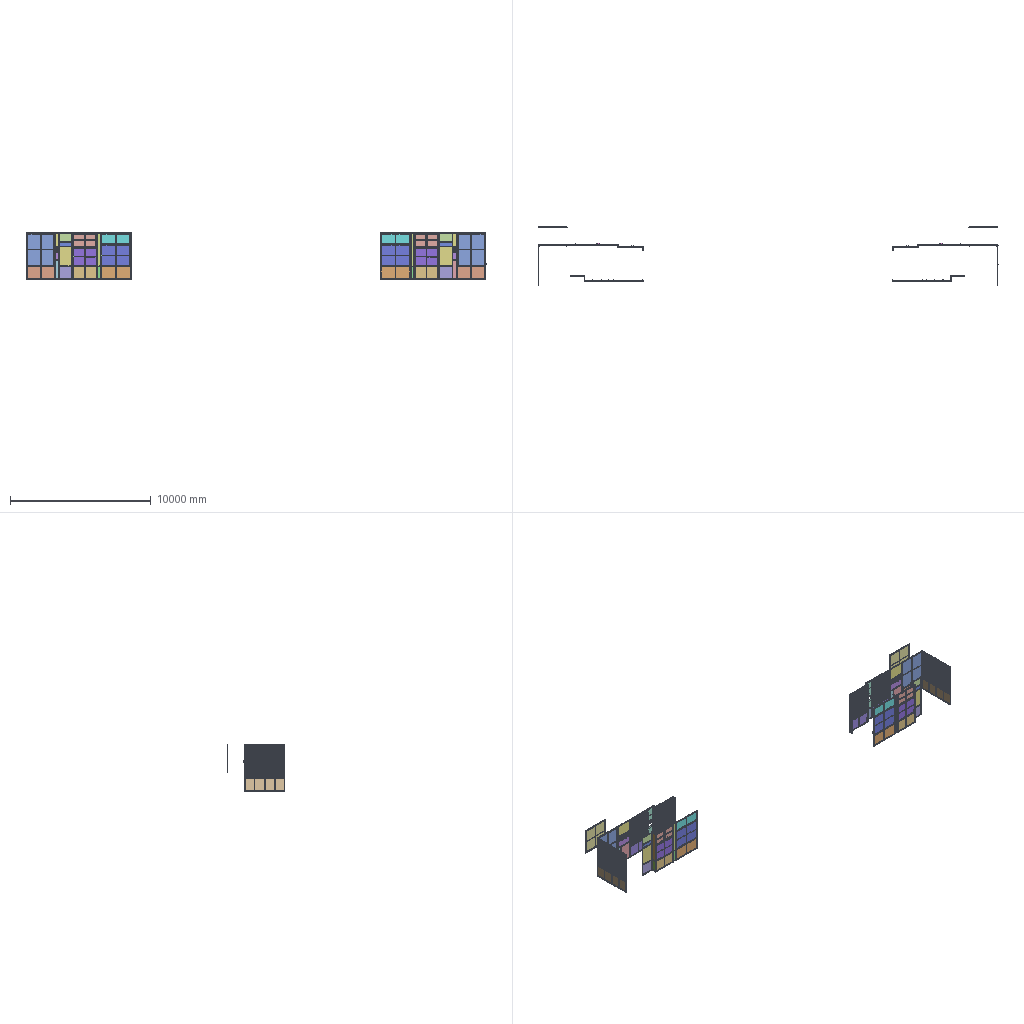Assembly | SolidWorks | 265 different items | 5997 placed | box 32704 x 4120 x 3280 mm
Parts list (item | name | quantity | parent item | size | volume | features):
1 | (subassembly) | x2 | in 40 | 1516 x 97 x 1065 mm | 8783731 mm3 | features ReferencePattern 4, CompositeCurve 1, DerivedHolePattern 1, LocalLPattern 1
2 | (subassembly) | x2 | in 40 | 722 x 54 x 1043 mm | 4219940 mm3 | features ReferencePattern 5, LocalLPattern 1
3 | (subassembly) | x2 | in 40 | 722 x 38 x 1043 mm | 4217360 mm3 | features ReferencePattern 5, LocalLPattern 1
4 | (subassembly) | x2 | - | - | - | -
5 | (subassembly) | x4 | in 4, 24 | - | 15054110 mm3 | features ReferencePattern 36, LocalLPattern 5, MirrorCompFeat 1
6 | (subassembly) | x4 | in 4, 24 | - | - | features ReferencePattern 178, LocalLPattern 10, MirrorCompFeat 4, CompositeCurve 1
7 | (subassembly) | x2 | - | - | 10335733 mm3 | features ReferencePattern 12, LocalLPattern 4
8 | (subassembly) | x2 | - | - | 7266370 mm3 | features ReferencePattern 12, LocalLPattern 4
9 | (subassembly) | x2 | - | - | 21498613 mm3 | -
10 | (subassembly) | x2 | in 9 | - | 21498613 mm3 | features ReferencePattern 30, LocalLPattern 10, MirrorCompFeat 1
11 | (subassembly) | x2 | - | - | 41950678 mm3 | -
12 | (subassembly) | x2 | in 11 | - | 17564416 mm3 | features ReferencePattern 19, LocalLPattern 3, DerivedHolePattern 2
13 | (subassembly) | x2 | in 11 | 2296 x 114.543 x 991.55 mm | 12200814 mm3 | features LocalLPattern 3, ReferencePattern 2, CompositeCurve 1
14 | (subassembly) | x2 | in 11 | 2296 x 97 x 991.55 mm | 12185495 mm3 | features LocalLPattern 2, ReferencePattern 1
15 | (subassembly) | x2 | - | - | 24877160 mm3 | -
16 | (subassembly) | x2 | in 15 | - | 5346170 mm3 | features ReferencePattern 13, DerivedHolePattern 3, LocalLPattern 2
17 | (subassembly) | x2 | in 15 | 1832 x 15 x 970 mm | 9765548 mm3 | features ReferencePattern 2, LocalLPattern 1
18 | (subassembly) | x2 | in 15 | 1832 x 15 x 970 mm | 9765539 mm3 | features ReferencePattern 2, LocalLPattern 1
19 | (subassembly) | x2 | - | - | 9752547 mm3 | -
20 | (subassembly) | x4 | - | - | 36484784 mm3 | -
21 | (subassembly) | x4 | in 20 | - | 13059635 mm3 | features ReferencePattern 57, LocalLPattern 5
22 | (subassembly) | x4 | in 20 | - | 23425150 mm3 | features ReferencePattern 138, LocalLPattern 9, MirrorCompFeat 4
23 | (subassembly) | x2 | - | - | 6905268 mm3 | features ReferencePattern 12, LocalLPattern 4
24 | (subassembly) | x2 | - | - | - | -
25 | (subassembly) | x2 | - | - | 7789967 mm3 | features ReferencePattern 12, LocalLPattern 4
26 | (subassembly) | x2 | - | - | 39443592 mm3 | -
27 | (subassembly) | x2 | in 26 | - | 16846770 mm3 | features ReferencePattern 45, LocalLPattern 6, MirrorCompFeat 5, CompositeCurve 3
28 | (subassembly) | x2 | in 19 | - | 7457075 mm3 | features ReferencePattern 8, LocalLPattern 2
29 | (subassembly) | x2 | in 26 | 1296 x 114.543 x 856.55 mm | 6140748 mm3 | features LocalLPattern 3, ReferencePattern 3, CompositeCurve 2
30 | (subassembly) | x2 | in 26 | 1296 x 97 x 857.775 mm | 6137895 mm3 | features LocalLPattern 2, ReferencePattern 2
31 | (subassembly) | x4 | in 26 | 852 x 78 x 956 mm | 5159135 mm3 | features ReferencePattern 28, LocalLPattern 5, MirrorCompFeat 2
32 | (subassembly) | x458 | in 5, 7, 8, 10, 12, 16, 21, 23, 25, 27, 28, 31, 39, 41 | 45.75 x 28.75 x 16 mm | 4951 mm3 | -
33 | (subassembly) | x1 | - | 46.643 x 46.639 x 38 mm | 6782 mm3 | -
34 | (subassembly) | x16 | in 31, 39 | 62 x 12.05 x 82 mm | 23876 mm3 | -
35 | (subassembly) | x16 | in 6 | 11 x 45 x 115 mm | 44302 mm3 | -
36 | (subassembly) | x1 | - | 69.2 x 20.1 x 100 mm | 14261 mm3 | -
37 | (subassembly) | x16 | in 16, 21, 41 | - | - | -
38 | (subassembly) | x2 | in 19 | 560.594 x 2339 x 38 mm | 2295468 mm3 | features ReferencePattern 12, LocalLPattern 3
39 | (subassembly) | x2 | - | - | 27416958 mm3 | features ReferencePattern 79, LocalLPattern 15, MirrorCompFeat 6, CompositeCurve 2
40 | (subassembly) | x2 | - | - | 46606535 mm3 | -
41 | (subassembly) | x2 | in 40 | - | 20597906 mm3 | features ReferencePattern 98, LocalLPattern 9
42 | (subassembly) | x2 | in 40 | 1516 x 114.543 x 1065 mm | 8787872 mm3 | features ReferencePattern 5, LocalLPattern 3, CompositeCurve 1
43 | - | x4 | in 6 | 160 x 64 x 4 mm | 39767 mm3 | features HoleWzd 2, Extrusion 1, Fillet 1
44 | - | x8 | in 12 | 14 x 20.3 x 907 mm | 46181 mm3 | features BaseBody 1, ICE 1, MoveFace 1
45 | - | x8 | in 8 | 14 x 20.3 x 95 mm | 4837 mm3 | features BaseBody 1, ICE 1, MoveFace 1
46 | - | x8 | in 41 | 14 x 20.3 x 980 mm | 49897 mm3 | features BaseBody 1, ICE 1, MoveFace 1
47 | - | x2 | in 29 | 30 x 15 x 1236 mm | 297813 mm3 | features HoleWzd 3, BaseBody 1, MoveFace 1
48 | - | x4 | in 29, 30 | 30 x 15 x 1236 mm | 297203 mm3 | features HoleWzd 3, BaseBody 1, MoveFace 1
49 | - | x2 | in 30 | 30 x 15 x 1236 mm | 297813 mm3 | features BaseBody 1, HoleWzd 1, MoveFace 1
50 | - | x4 | in 1, 42 | 30 x 15 x 1456 mm | 350164 mm3 | features HoleWzd 3, BaseBody 1, MoveFace 1
51 | - | x4 | in 1, 42 | 30 x 15 x 1456 mm | 351142 mm3 | features BaseBody 1, HoleWzd 1, MoveFace 1
52 | - | x4 | in 17, 18 | 30 x 15 x 1772 mm | 426374 mm3 | features HoleWzd 3, BaseBody 1, MoveFace 1
53 | - | x4 | in 17, 18 | 30 x 15 x 1772 mm | 427079 mm3 | features BaseBody 1, HoleWzd 1, MoveFace 1
54 | - | x8 | in 6 | 40 x 40 x 4 mm | 5920 mm3 | features HoleWzd 3, Extrusion 1, Fillet 1
55 | - | x4 | in 13, 14 | 30 x 15 x 2236 mm | 538276 mm3 | features HoleWzd 3, BaseBody 1, MoveFace 1
56 | - | x1 | - | 30 x 15 x 2236 mm | 538276 mm3 | features HoleWzd 3, BaseBody 1, MoveFace 1
57 | - | x1 | - | 30 x 15 x 2236 mm | 538276 mm3 | features HoleWzd 3, BaseBody 1, MoveFace 1
58 | - | x1 | - | 30 x 15 x 2236 mm | 538710 mm3 | features BaseBody 1, HoleWzd 1, MoveFace 1
59 | - | x4 | in 13, 14 | 30 x 15 x 2236 mm | 538982 mm3 | features BaseBody 1, HoleWzd 1, MoveFace 1
60 | - | x1 | - | 30 x 15 x 630 mm | 151936 mm3 | features BaseBody 1, MoveFace 1
61 | - | x4 | in 2, 3 | 30 x 15 x 662 mm | 159462 mm3 | features BaseBody 1, HoleWzd 1, MoveFace 1
62 | - | x4 | in 2, 3 | 30 x 15 x 662 mm | 159654 mm3 | features BaseBody 1, MoveFace 1
63 | - | x12 | in 29, 30 | 30 x 15 x 775 mm | 186906 mm3 | features BaseBody 1, MoveFace 1
64 | - | x1 | - | 30 x 15 x 791 mm | 190764 mm3 | features BaseBody 1, MoveFace 1
65 | - | x12 | in 12, 27, 41 | 45 x 26 x 108 mm | 14308 mm3 | features HoleWzd 2, Fillet 1, FlatPattern 1, SMBaseFlange 1, SheetMetal 1
66 | - | x4 | in 13, 14 | 30 x 15 x 910 mm | 219062 mm3 | features BaseBody 1, HoleWzd 1, MoveFace 1
67 | - | x20 | in 13, 14, 17, 18 | 30 x 15 x 910 mm | 219464 mm3 | features BaseBody 1, MoveFace 1
68 | - | x20 | in 1, 2, 3, 42 | 30 x 15 x 983 mm | 237069 mm3 | features BaseBody 1, MoveFace 1
69 | - | x4 | in 39 | 40 x 40 x 1350 mm | 790915 mm3 | features BaseBody 1, HoleWzd 1, MoveFace 1
70 | - | x20 | in 5, 21, 24 | 40 x 40 x 3280 mm | 1969669 mm3 | features HoleWzd 2, Extrusion 1
71 | - | x8 | in 39 | 40 x 40 x 1146 mm | 670131 mm3 | features BaseBody 1, HoleWzd 1, MoveFace 1
72 | - | x6 | in 23 | 40 x 40 x 135 mm | 71545 mm3 | features BaseBody 1, HoleWzd 1, MoveFace 1
73 | - | x4 | in 21 | 40 x 40 x 1360 mm | 796835 mm3 | features BaseBody 1, HoleWzd 1, MoveFace 1
74 | - | x6 | in 8 | 40 x 40 x 155 mm | 83386 mm3 | features BaseBody 1, HoleWzd 1, MoveFace 1
75 | - | x8 | in 27 | 40 x 40 x 1650 mm | 968537 mm3 | features BaseBody 1, HoleWzd 1, MoveFace 1
76 | - | x6 | in 1, 14, 30 | 52 x 17 x 50 mm | 6238 mm3 | features HoleWzd 2, Fillet 1, FlatPattern 1, SMBaseFlange 1, SheetMetal 1
77 | - | x4 | in 5 | 40 x 40 x 1682 mm | 987483 mm3 | features BaseBody 1, HoleWzd 1, MoveFace 1
78 | - | x6 | in 25 | 40 x 40 x 184 mm | 100557 mm3 | features BaseBody 1, HoleWzd 1, MoveFace 1
79 | - | x10 | in 12, 16 | 40 x 40 x 1920 mm | 1128397 mm3 | features BaseBody 1, HoleWzd 1, MoveFace 1
80 | - | x2 | in 39 | 40 x 40 x 1930 mm | 1139883 mm3 | features HoleWzd 4, MoveFace 2, BaseBody 1
81 | - | x4 | in 16 | 40 x 40 x 1930 mm | 1140355 mm3 | features HoleWzd 3, BaseBody 1, MoveFace 1
82 | - | x8 | in 41 | 40 x 40 x 2066 mm | 1214839 mm3 | features BaseBody 1, HoleWzd 1, MoveFace 1
83 | - | x2 | in 39 | 40 x 40 x 308 mm | 173974 mm3 | features BaseBody 1, HoleWzd 1, MoveFace 1
84 | - | x6 | in 7 | 40 x 40 x 325 mm | 184039 mm3 | features BaseBody 1, HoleWzd 1, MoveFace 1
85 | - | x24 | in 7, 8, 23, 25, 28, 41 | 40 x 40 x 3280 mm | 1939169 mm3 | features HoleWzd 4, 3DProfileFeature 1, BaseBody 1, MoveFace 1
86 | - | x2 | in 39 | 40 x 40 x 3280 mm | 1938394 mm3 | features HoleWzd 4, BaseBody 1, MoveFace 1
87 | - | x6 | in 13, 29, 42 | 68 x 17 x 50 mm | 7802 mm3 | features HoleWzd 2, Fillet 1, FlatPattern 1, SMBaseFlange 1, SheetMetal 1
88 | - | x2 | in 27 | 40 x 40 x 3280 mm | 1938394 mm3 | features HoleWzd 6, BaseBody 1, MoveFace 1
89 | - | x2 | in 27 | 40 x 40 x 3280 mm | 1938394 mm3 | features HoleWzd 6, BaseBody 1, MoveFace 1
90 | - | x4 | in 12 | 40 x 40 x 3280 mm | 1940425 mm3 | features HoleWzd 2, BaseBody 1, MoveFace 1
91 | - | x6 | in 28 | 40 x 40 x 536 mm | 308966 mm3 | features BaseBody 1, HoleWzd 1, MoveFace 1
92 | - | x2 | in 39 | 40 x 40 x 798 mm | 464090 mm3 | features BaseBody 1, HoleWzd 1, MoveFace 1
93 | - | x14 | in 5, 12, 21, 27, 41 | 40 x 40 x 846 mm | 492509 mm3 | features BaseBody 1, HoleWzd 1, MoveFace 1
94 | - | x10 | in 10 | 40 x 40 x 880 mm | 512640 mm3 | features BaseBody 1, HoleWzd 1, MoveFace 1
95 | - | x8 | in 39 | 40 x 40 x 339 mm | 146697 mm3 | features BaseBody 1, MoveFace 1
96 | - | x12 | in 39 | 40 x 40 x 488 mm | 205502 mm3 | features BaseBody 1, HoleWzd 1, MoveFace 1
97 | - | x12 | in 31 | 40 x 40 x 740 mm | 314551 mm3 | features BaseBody 1, HoleWzd 1, MoveFace 1
98 | - | x8 | in 27, 39 | 70 x 54 x 82 mm | 19533 mm3 | features HoleWzd 3, EdgeFlange 2, Chamfer 1, Fillet 1, FlatPattern 1, MirrorPattern 1, SMBaseFlange 1, SheetMetal 1
99 | - | x8 | in 31 | 40 x 40 x 956 mm | 413693 mm3 | features BaseBody 1, MoveFace 1
100 | - | x8 | in 21 | 40 x 40 x 1360 mm | 721762 mm3 | features BaseBody 1, HoleWzd 1, MoveFace 1
101 | - | x1 | - | 40 x 40 x 155 mm | 83065 mm3 | features BaseBody 1, HoleWzd 1, MoveFace 1
102 | - | x8 | in 5 | 40 x 40 x 1682 mm | 894323 mm3 | features BaseBody 1, HoleWzd 1, MoveFace 1
103 | - | x1 | - | 40 x 40 x 1762 mm | 942816 mm3 | features BaseBody 1, HoleWzd 1, MoveFace 1
104 | - | x1 | - | 40 x 40 x 2150 mm | 1150023 mm3 | features BaseBody 1, HoleWzd 1, MoveFace 1
105 | - | x1 | - | 40 x 40 x 2154 mm | 1154336 mm3 | features BaseBody 1, HoleWzd 1, MoveFace 1
106 | - | x32 | in 6, 22 | 40 x 40 x 2310 mm | 1236491 mm3 | features BaseBody 1
107 | - | x1 | - | 40 x 40 x 255 mm | 136655 mm3 | features BaseBody 1, HoleWzd 1, MoveFace 1
108 | - | x4 | in 10 | 40 x 40 x 3280 mm | 1939269 mm3 | features HoleWzd 3, BaseBody 1, MoveFace 1
109 | - | x8 | in 27, 39 | 42 x 25 x 50 mm | 6162 mm3 | features HoleWzd 3, EdgeFlange 2, Chamfer 1, Fillet 1, FlatPattern 1, MirrorPattern 1, SMBaseFlange 1, SheetMetal 1
110 | - | x8 | in 22 | 40 x 40 x 588 mm | 315111 mm3 | features BaseBody 1, MoveFace 1
111 | - | x20 | in 22 | 40 x 40 x 588 mm | 315111 mm3 | features BaseBody 1, MoveFace 1
112 | - | x28 | in 6 | 40 x 40 x 749 mm | 401392 mm3 | features BaseBody 1, MoveFace 1
113 | - | x1 | - | 40 x 40 x 757 mm | 405679 mm3 | features BaseBody 1, MoveFace 1
114 | - | x16 | in 22 | 60 x 38 x 3 mm | 6476 mm3 | features BaseBody 1
115 | - | x32 | in 35 | 45 x 11 x 113 mm | 18493 mm3 | features BaseBody 1
116 | - | x16 | in 35 | 9 x 9 x 115 mm | 7316 mm3 | features BaseBody 1
117 | - | x160 | in 1, 2, 3, 13, 14, 17, 18, 29, 30, 42 | 10.5 x 10.5 x 19.3 mm | 617.652 mm3 | features BaseBody 1
118 | - | x4 | in 27 | 11.6 x 1.2 x 11.6 mm | 88.216 mm3 | features Extrusion 1
119 | - | x8 | in 41 | 17.5 x 34 x 40 mm | 3554 mm3 | features HoleWzd 2, Fillet 1, FlatPattern 1, SMBaseFlange 1, SheetMetal 1
120 | - | x40 | in 12, 16, 27, 41 | 7 x 7 x 0.5 mm | 15.221 mm3 | features Revolution 1
121 | - | x16 | in 2, 3 | 9 x 9 x 0.8 mm | 39.276 mm3 | features Revolution 1
122 | - | x124 | in 5, 12, 16, 21, 27, 41 | 10 x 10 x 1 mm | 56.478 mm3 | features Revolution 1
123 | - | x32 | in 22 | 12.5 x 12.5 x 1.6 mm | 144.878 mm3 | features Revolution 1
124 | - | x96 | in 6 | 15 x 8.5 x 20 mm | 1520 mm3 | features BaseBody 1
125 | - | x32 | in 22 | 12.197 x 12.2 x 1.5 mm | 128.674 mm3 | features ICE 1, Revolution 1
126 | - | x8 | in 31, 39 | 107 x 38 x 20.5 mm | 23344 mm3 | features BaseBody 1
127 | - | x12 | in 12, 27, 41 | - | - | features BaseBody 30, RefSurface 1
128 | - | x12 | in 1, 13, 14, 29, 30, 42 | 35.586 x 51.386 x 50.3 mm | 17360 mm3 | features BaseBody 15
129 | - | x4 | in 41 | 1009 x 842 x 5 mm | 4247890 mm3 | features Extrusion 1, HoleWzd 1
130 | - | x2 | in 38 | 533 x 2311 x 38 mm | 2271037 mm3 | features SMWeldBead 4, EdgeFlange 2, HoleWzd 2, BossThin 1, FlatPattern 1, ICE 1, SMBaseFlange 1, SheetMetal 1
131 | - | x16 | in 22 | 584 x 1091 x 5 mm | 3185720 mm3 | features Extrusion 1, HoleWzd 1
132 | - | x16 | in 6 | 745 x 1091 x 5 mm | 4063975 mm3 | features Extrusion 1, HoleWzd 1
133 | - | x1 | - | 646 x 1119 x 5 mm | 3614370 mm3 | features Extrusion 1
134 | - | x1 | - | 807 x 1119 x 5 mm | 4515165 mm3 | features Extrusion 1
135 | - | x8 | in 13, 14 | 926 x 1119 x 5 mm | 5180970 mm3 | features Extrusion 1
136 | - | x2 | in 39 | 1142 x 513 x 5 mm | 2929230 mm3 | features Extrusion 1, HoleWzd 1
137 | - | x2 | in 39 | 1142 x 906 x 5 mm | 5173260 mm3 | features Extrusion 1, HoleWzd 1
138 | - | x2 | in 23 | 131 x 2310 x 5 mm | 1513050 mm3 | features Extrusion 1, HoleWzd 1
139 | - | x2 | in 23 | 131 x 842 x 5 mm | 551510 mm3 | features Extrusion 1, HoleWzd 1
140 | - | x2 | in 8 | 151 x 2310 x 5 mm | 1744050 mm3 | features Extrusion 1, HoleWzd 1
141 | - | x16 | in 6 | 1144 x 813 x 7 mm | 815811 mm3 | features ICE 5, Extrusion 1, HoleWzd 1, WeldmentFeature 1
142 | - | x2 | in 8 | 151 x 842 x 5 mm | 635710 mm3 | features Extrusion 1, HoleWzd 1
143 | - | x2 | in 25 | 180 x 2310 x 5 mm | 2079000 mm3 | features Extrusion 1, HoleWzd 1
144 | - | x2 | in 25 | 180 x 842 x 5 mm | 757800 mm3 | features Extrusion 1, HoleWzd 1
145 | - | x2 | in 39 | 304 x 1306 x 5 mm | 1985120 mm3 | features Extrusion 1, HoleWzd 1
146 | - | x2 | in 7 | 321 x 2310 x 5 mm | 3707550 mm3 | features Extrusion 1, HoleWzd 1
147 | - | x2 | in 7 | 321 x 842 x 5 mm | 1351410 mm3 | features Extrusion 1, HoleWzd 1
148 | - | x8 | in 39 | 484 x 105 x 5 mm | 254100 mm3 | features Extrusion 1, HoleWzd 1
149 | - | x2 | in 28 | 532 x 842 x 5 mm | 2239720 mm3 | features Extrusion 1, HoleWzd 1
150 | - | x8 | in 29, 30 | 619 x 791 x 5 mm | 2448145 mm3 | features Extrusion 1
151 | - | x8 | in 21 | 656 x 842 x 5 mm | 2761760 mm3 | features Extrusion 1, HoleWzd 1
152 | - | x16 | in 22 | 1143 x 652 x 7 mm | 701424 mm3 | features ICE 5, Extrusion 1, HoleWzd 1, WeldmentFeature 1
153 | - | x4 | in 2, 3 | 997 x 678 x 5 mm | 3379830 mm3 | features Extrusion 1
154 | - | x8 | in 31 | 414 x 736 x 5 mm | 1523520 mm3 | features Extrusion 1, HoleWzd 1
155 | - | x2 | in 39 | 794 x 1306 x 5 mm | 5184820 mm3 | features Extrusion 1, HoleWzd 1
156 | - | x4 | in 27 | 801 x 842 x 5 mm | 3372210 mm3 | features Extrusion 1, HoleWzd 1
157 | - | x8 | in 5 | 817 x 842 x 5 mm | 3439570 mm3 | features Extrusion 1, HoleWzd 1
158 | - | x2 | in 10 | 876 x 1360 x 5 mm | 5956800 mm3 | features Extrusion 1, HoleWzd 1
159 | - | x2 | in 10 | 876 x 291 x 5 mm | 1274580 mm3 | features Extrusion 1, HoleWzd 1
160 | - | x2 | in 10 | 876 x 571 x 5 mm | 2500980 mm3 | features Extrusion 1, HoleWzd 1
161 | - | x2 | in 10 | 876 x 842 x 5 mm | 3687960 mm3 | features Extrusion 1, HoleWzd 1
162 | - | x8 | in 17, 18 | 926 x 887 x 5 mm | 4106810 mm3 | features Extrusion 1
163 | - | x8 | in 27, 39 | 16.002 x 50.042 x 18.313 mm | 6537 mm3 | features BaseBody 8
164 | - | x4 | in 12 | 936 x 842 x 5 mm | 3940560 mm3 | features Extrusion 1, HoleWzd 1
165 | - | x8 | in 1, 42 | 999 x 729 x 5 mm | 3641355 mm3 | features Extrusion 1
166 | - | x4 | in 27 | 10 x 4.5 x 6 mm | 142.178 mm3 | features ICE 2, Extrusion 1, Fillet 1, RevCut 1
167 | - | x4 | in 27 | 19 x 7.5 x 7.999 mm | 677.198 mm3 | features ICE 2, Extrusion 1, RevCut 1
168 | - | x12 | in 1, 13, 14, 29, 30, 42 | 18 x 135 x 30 mm | 20354 mm3 | features BaseBody 1
169 | - | x12 | in 14, 29, 30 | 8 x 8 x 20 mm | 286.49 mm3 | features BaseBody 1
170 | - | x40 | in 1, 2, 3, 13, 14, 17, 18, 29, 30, 42 | 32 x 32 x 15 mm | 8367 mm3 | features BaseBody 1
171 | - | x26 | in 6, 27, 39 | 55 x 14.5 x 18 mm | 8175 mm3 | features BaseBody 1
172 | - | x20 | in 12, 16, 27, 41 | 17 x 15 x 50 mm | 8082 mm3 | features BaseBody 1
173 | - | x4 | in 6 | 16.3 x 18.3 x 16.3 mm | 1833 mm3 | features BaseBody 1
174 | - | x8 | in 27, 39 | 16.008 x 126.481 x 28.318 mm | 9351 mm3 | features BaseBody 7
175 | - | x1 | - | 8 x 1328 x 777 mm | 322628 mm3 | features BaseBody 1, ICE 1, MirrorPattern 1
176 | - | x1 | - | 8 x 742 x 777 mm | 178056 mm3 | features BaseBody 1, ICE 1, MirrorPattern 1
177 | - | x4 | in 27 | 33.5 x 13.5 x 1650 mm | 308881 mm3 | features BaseBody 1, HoleWzd 1, ICE 1, MoveFace 1
178 | - | x4 | in 12 | 33.5 x 13.5 x 1920 mm | 359220 mm3 | features ICE 2, BaseBody 1, HoleWzd 1, MoveFace 1
179 | - | x4 | in 16 | 33.5 x 13.5 x 1920 mm | 359220 mm3 | features ICE 2, BaseBody 1, HoleWzd 1, MoveFace 1
180 | - | x4 | in 6 | - | 237710 mm3 | features BaseBody 17, ICE 1
181 | - | x8 | in 41 | 33.5 x 13.5 x 2066 mm | 386658 mm3 | features ICE 2, BaseBody 1, HoleWzd 1, MoveFace 1
182 | - | x40 | in 1, 2, 3, 13, 14, 17, 18, 29, 30, 42 | 32 x 32 x 15 mm | 8036 mm3 | features BaseBody 1
183 | - | x4 | in 6 | - | 135185 mm3 | features BaseBody 17
184 | - | x8 | in 10 | 13.8 x 7.5 x 8 mm | 622.996 mm3 | features BaseBody 1
185 | - | x260 | in 5, 6, 12, 21, 22, 27, 39, 41 | 19.5 x 6 x 8 mm | 667.11 mm3 | features BaseBody 1
186 | - | x550 | in 5, 12, 21, 31, 32, 39, 41 | 19.5 x 6 x 8 mm | 631.457 mm3 | features BaseBody 1
187 | - | x174 | in 5, 7, 8, 10, 12, 16, 21, 23, 25, 28, 31, 38, 39, 41 | 13.001 x 8.797 x 21 mm | 1304 mm3 | features BaseBody 1
188 | - | x1 | - | - | - | features RefSurface 120
189 | - | x1 | - | 41 x 41 x 38 mm | 6489 mm3 | features BaseBody 1
190 | - | x16 | in 34 | 36.75 x 12.05 x 79 mm | 10360 mm3 | features BaseBody 1
191 | - | x16 | in 34 | 7 x 7 x 82 mm | 3156 mm3 | features BaseBody 1
192 | - | x16 | in 34 | 36.75 x 12.05 x 79 mm | 10360 mm3 | features BaseBody 1
193 | - | x1 | - | 69.2 x 20 x 100 mm | 10290 mm3 | features BaseBody 1
194 | - | x1 | - | 69.2 x 7 x 25.2 mm | 3971 mm3 | features BaseBody 1
195 | - | x2 | in 39 | 9.5 x 13.5 x 140 mm | 13278 mm3 | features BaseBody 1
196 | - | x120 | in 5, 12, 16, 21, 27, 41 | 5.5 x 6.351 x 2.4 mm | 50.752 mm3 | features BaseBody 1
197 | - | x56 | in 12, 16, 27, 41 | 7 x 8.083 x 3.2 mm | 107.56 mm3 | features BaseBody 1
198 | - | x2 | in 27 | 8 x 9.238 x 4 mm | 165.049 mm3 | features BaseBody 1
199 | - | x1 | - | 39 x 25 x 60 mm | 7010 mm3 | features HoleWzd 2, Chamfer 1, FlatPattern 1, SMBaseFlange 1, SheetMetal 1
200 | - | x40 | in 12, 16, 27, 41 | 5.5 x 5.5 x 11 mm | 117.558 mm3 | features ICE 2, Chamfer 1, RevCut 1, Revolution 1
201 | - | x16 | in 41 | 7 x 7 x 16 mm | 285.079 mm3 | features ICE 2, Chamfer 1, RevCut 1, Revolution 1
202 | - | x80 | in 1, 2, 3, 13, 14, 29, 30, 42 | 7 x 7 x 12 mm | 234.462 mm3 | features ICE 3, Chamfer 1, RevCut 1, Revolution 1
203 | - | x292 | in 5, 6, 12, 16, 21, 27, 39, 41 | 17 x 8.5 x 8.5 mm | 477.486 mm3 | features ICE 1, RevCut 1, Revolution 1
204 | - | x24 | in 38 | 18 x 10 x 10 mm | 732.461 mm3 | features ICE 1, RevCut 1, Revolution 1
205 | - | x32 | in 22 | 22 x 10 x 10 mm | 845.558 mm3 | features ICE 1, RevCut 1, Revolution 1
206 | - | x16 | in 31, 39 | 10 x 10 x 24 mm | 898.677 mm3 | features Chamfer 2, ICE 2, RevCut 1, Revolution 1
207 | - | x16 | in 13, 14, 17, 18 | 10 x 10 x 36 mm | 1238 mm3 | features Chamfer 2, ICE 2, RevCut 1, Revolution 1
208 | - | x124 | in 5, 7, 8, 10, 12, 16, 21, 23, 25, 28, 39, 41 | 10 x 10 x 46 mm | 1521 mm3 | features Chamfer 2, ICE 2, RevCut 1, Revolution 1
209 | - | x72 | in 6, 22 | 13 x 13 x 48 mm | 2916 mm3 | features Chamfer 2, ICE 2, RevCut 1, Revolution 1
210 | - | x1 | - | 23 x 25 x 60 mm | 5085 mm3 | features HoleWzd 2, Chamfer 1, FlatPattern 1, SMBaseFlange 1, SheetMetal 1
211 | - | x40 | in 12, 16, 27, 41 | 8 x 8 x 10 mm | 162.002 mm3 | features BaseBody 1
212 | - | x1 | - | 10 x 10 x 12 mm | 304.022 mm3 | features BaseBody 1
213 | - | x48 | in 31, 39 | 12 x 12 x 15 mm | 531.654 mm3 | features BaseBody 1
214 | - | x48 | in 31, 39 | 12 x 12 x 25 mm | 814.397 mm3 | features BaseBody 1
215 | - | x212 | in 5, 6, 12, 16, 21, 22, 27, 41 | 12 x 12 x 12 mm | 460.573 mm3 | features Chamfer 1, ICE 1, Revolution 1
216 | - | x8 | in 27 | 17 x 8.5 x 8.5 mm | 492.043 mm3 | features ICE 1, Revolution 1
217 | - | x458 | in 32 | 10 x 10 x 31 mm | 1100 mm3 | features BaseBody 1
218 | - | x1 | - | 38 x 31 x 14.5 mm | 4841 mm3 | features BaseBody 1
219 | - | x8 | in 25 | 10.8 x 17.5 x 124 mm | 9771 mm3 | features MoveFace 2, BaseBody 1
220 | - | x4 | in 10 | 10.8 x 17.5 x 1358 mm | 107011 mm3 | features BaseBody 1, MoveFace 1
221 | - | x18 | in 2, 29, 42 | 39 x 17 x 40 mm | 4045 mm3 | features HoleWzd 2, FlatPattern 1, SMBaseFlange 1, SheetMetal 1
222 | - | x16 | in 7, 8, 23, 25 | 10.8 x 17.5 x 1171 mm | 92275 mm3 | features BaseBody 1, MoveFace 1
223 | - | x8 | in 7 | 10.8 x 17.5 x 265 mm | 20882 mm3 | features BaseBody 1, MoveFace 1
224 | - | x4 | in 28 | 10.8 x 17.5 x 476 mm | 37509 mm3 | features BaseBody 1, MoveFace 1
225 | - | x16 | in 21 | 10.8 x 17.5 x 627 mm | 49408 mm3 | features BaseBody 1, MoveFace 1
226 | - | x8 | in 23 | 10.8 x 17.5 x 75 mm | 5910 mm3 | features BaseBody 1, MoveFace 1
227 | - | x8 | in 27 | 10.8 x 17.5 x 774 mm | 60992 mm3 | features BaseBody 1, MoveFace 1
228 | - | x24 | in 5, 12, 21, 41 | 10.8 x 17.5 x 786 mm | 61937 mm3 | features BaseBody 1, MoveFace 1
229 | - | x24 | in 5, 27 | 10.8 x 17.5 x 788 mm | 62095 mm3 | features BaseBody 1, MoveFace 1
230 | - | x16 | in 10 | 10.8 x 17.5 x 820 mm | 64616 mm3 | features BaseBody 1, MoveFace 1
231 | - | x48 | in 5, 7, 8, 10, 12, 21, 23, 25, 28, 41 | 10.8 x 17.5 x 840 mm | 66192 mm3 | features BaseBody 1, MoveFace 1
232 | - | x20 | in 12, 16, 27, 41 | 17.5 x 17 x 60 mm | 3562 mm3 | features HoleWzd 2, FlatPattern 1, SMBaseFlange 1, SheetMetal 1
233 | - | x8 | in 12 | 10.8 x 17.5 x 907 mm | 71472 mm3 | features BaseBody 1, MoveFace 1
234 | - | x8 | in 8 | 10.8 x 17.5 x 95 mm | 7486 mm3 | features MoveFace 2, BaseBody 1
235 | - | x8 | in 41 | 10.8 x 17.5 x 980 mm | 77225 mm3 | features BaseBody 1, MoveFace 1
236 | - | x8 | in 7 | 14 x 20.3 x 265 mm | 13493 mm3 | features MoveFace 2, BaseBody 1, ICE 1
237 | - | x8 | in 39 | 14 x 20.3 x 1088 mm | 55396 mm3 | features BaseBody 1, ICE 1, MoveFace 1
238 | - | x16 | in 39 | 14 x 20.3 x 108 mm | 5499 mm3 | features MoveFace 2, BaseBody 1, ICE 1
239 | - | x64 | in 6, 22 | 14 x 20.3 x 1090 mm | 55498 mm3 | features BaseBody 1, ICE 1, MoveFace 1
240 | - | x8 | in 25 | 14 x 20.3 x 124 mm | 6314 mm3 | features BaseBody 1, ICE 1, MoveFace 1
241 | - | x8 | in 39 | 14 x 20.3 x 1280 mm | 65172 mm3 | features BaseBody 1, ICE 1, MoveFace 1
242 | - | x4 | in 10 | 14 x 20.3 x 1358 mm | 69144 mm3 | features BaseBody 1, ICE 1, MoveFace 1
243 | - | x12 | in 1, 3, 14, 30 | 23 x 17 x 40 mm | 2765 mm3 | features HoleWzd 2, FlatPattern 1, SMBaseFlange 1, SheetMetal 1
244 | - | x16 | in 7, 8, 23, 25 | 14 x 20.3 x 2314 mm | 117819 mm3 | features BaseBody 1, ICE 1, MoveFace 1
245 | - | x4 | in 39 | 14 x 20.3 x 251 mm | 12780 mm3 | features MoveFace 2, BaseBody 1, ICE 1
246 | - | x6 | in 10 | 14 x 20.3 x 291 mm | 14816 mm3 | features MoveFace 2, BaseBody 1, ICE 1
247 | - | x16 | in 31 | 14 x 20.3 x 413 mm | 21028 mm3 | features BaseBody 1, ICE 1, MoveFace 1
248 | - | x16 | in 39 | 14 x 20.3 x 430 mm | 21894 mm3 | features BaseBody 1, ICE 1, MoveFace 1
249 | - | x4 | in 28 | 14 x 20.3 x 476 mm | 24236 mm3 | features BaseBody 1, ICE 1, MoveFace 1
250 | - | x4 | in 39 | 14 x 20.3 x 513 mm | 26120 mm3 | features BaseBody 1, ICE 1, MoveFace 1
251 | - | x32 | in 22 | 14 x 20.3 x 528 mm | 26884 mm3 | features BaseBody 1, ICE 1, MoveFace 1
252 | - | x4 | in 10 | 14 x 20.3 x 571 mm | 29073 mm3 | features MoveFace 2, BaseBody 1, ICE 1
253 | - | x16 | in 21 | 14 x 20.3 x 627 mm | 31924 mm3 | features BaseBody 1, ICE 1, MoveFace 1
254 | - | x24 | in 5, 27, 39 | 72 x 17 x 32 mm | 6272 mm3 | features Chamfer 1, FlatPattern 1, HoleWzd 1, SMBaseFlange 1, SheetMetal 1
255 | - | x16 | in 31 | 14 x 20.3 x 680 mm | 34623 mm3 | features BaseBody 1, ICE 1, MoveFace 1
256 | - | x32 | in 6 | 14 x 20.3 x 689 mm | 35081 mm3 | features BaseBody 1, ICE 1, MoveFace 1
257 | - | x4 | in 39 | 14 x 20.3 x 740 mm | 37678 mm3 | features BaseBody 1, ICE 1, MoveFace 1
258 | - | x8 | in 23 | 14 x 20.3 x 75 mm | 3819 mm3 | features BaseBody 1, ICE 1, MoveFace 1
259 | - | x8 | in 27 | 14 x 20.3 x 774 mm | 39409 mm3 | features BaseBody 1, ICE 1, MoveFace 1
260 | - | x24 | in 5, 12, 21, 41 | 14 x 20.3 x 786 mm | 40020 mm3 | features BaseBody 1, ICE 1, MoveFace 1
261 | - | x24 | in 5, 27 | 14 x 20.3 x 788 mm | 40122 mm3 | features BaseBody 1, ICE 1, MoveFace 1
262 | - | x16 | in 10 | 14 x 20.3 x 820 mm | 41751 mm3 | features BaseBody 1, ICE 1, MoveFace 1
263 | - | x48 | in 5, 7, 8, 10, 12, 21, 23, 25, 28, 41 | 14 x 20.3 x 840 mm | 42769 mm3 | features BaseBody 1, ICE 1, MoveFace 1
264 | - | x4 | in 39 | 14 x 20.3 x 906 mm | 46130 mm3 | features BaseBody 1, ICE 1, MoveFace 1
265 | - | x458 | in 32 | 28 x 18.5 x 16 mm | 3220 mm3 | features BaseBody 1
Mates (type | each side: item.copy, entity, surface, feature), first 382 of 2353 lines:
In the top assembly
Coincident | 85.1 face plane 输入1 | assembly face | 3 times
Coincident | 85.1 face plane 输入1 | 70.1 face plane Boss-Extrude 1 | 3 times
Coincident | 85.2 face plane 输入1 | 85.3 face plane 输入1 | 3 times
Coincident | 69.1 face plane 输入1 | 90.1 face plane 输入1
Coincident | 86.1 face plane 输入1 | 70.2 face plane Boss-Extrude 1 | 3 times
Coincident | 80.1 face plane 输入1 | 90.1 face plane 输入1 | 2 times
Coincident | 86.1 face plane 输入1 | assembly face | 3 times
Coincident | 88.1 face plane 输入1 | 85.4 face plane 输入1 | 6 times
Coincident | 85.5 face plane 输入1 | 89.1 face plane 输入1 | 6 times
Coincident | 85.6 face plane 输入1 | 75.1 face plane 输入1
Coincident | 85.6 face plane 输入1 | 89.2 face plane 输入1 | 2 times
Coincident | 85.7 face plane 输入1 | 108.1 face plane 输入1 | 2 times
Coincident | 84.1 face plane 输入1 | 94.1 face plane 输入1
Coincident | 85.8 face plane 输入1 | 89.2 face plane 输入1
Coincident | 85.8 face plane 输入1 | 75.1 face plane 输入1
Coincident | 85.8 face plane 输入1 | 88.2 face plane 输入1
Coincident | 85.9 face plane 输入1 | 85.10 face plane 输入1 | 3 times
Coincident | 90.2 face plane 输入1 | 70.3 face plane Boss-Extrude 1 | 3 times
Coincident | 86.2 face plane 输入1 | 90.3 face plane 输入1 | 3 times
Coincident | 79.1 face plane 输入1 | 79.2 face plane 输入1
Coincident | 90.2 face plane 输入1 | 81.1 face plane 输入1
Coincident | 69.2 face plane 输入1 | assembly face
Coincident | 69.2 face plane 输入1 | 70.4 face plane Boss-Extrude 1 | 3 times
Coincident | 80.2 face plane 输入1 | assembly face | 2 times
Coincident | 85.11 face plane 输入1 | 85.12 face plane 输入1 | 3 times
Coincident | 85.13 face plane 输入1 | 108.2 face plane 输入1 | 3 times
Coincident | 85.14 face plane 输入1 | 70.5 face plane Boss-Extrude 1 | 3 times
Coincident | 90.4 face plane 输入1 | 70.6 face plane Boss-Extrude 1 | 3 times
Coincident | 79.3 face plane 输入1 | 79.4 face plane 输入1
DistanceDim | 81.2 face plane 输入1 | 90.4 face plane 输入1
Coincident | 90.4 face plane 输入1 | 81.2 face plane 输入1
Coincident | 70.7 face plane Boss-Extrude 1 | 70.8 face plane Boss-Extrude 1 | 3 times
Coincident | 85.15 face plane 输入1 | 70.9 face plane Boss-Extrude 1 | 3 times
Coincident | 85.15 face plane 输入1 | assembly face | 3 times
Coincident | 85.16 face plane 输入1 | 70.10 face plane Boss-Extrude 1 | 3 times
Coincident | 85.17 face plane 输入1 | 70.11 face plane Boss-Extrude 1 | 3 times
Coincident | 85.17 face plane 输入1 | assembly face | 4 times
Coincident | 70.12 face plane Boss-Extrude 1 | 70.13 face plane Boss-Extrude 1 | 3 times
Coincident | 85.18 face plane 输入1 | 70.14 face plane Boss-Extrude 1 | 3 times
Coincident | 85.18 face plane 输入1 | assembly face | 4 times
Coincident | 85.19 face plane 输入1 | 85.20 face plane 输入1 | 5 times
Coincident | 81.3 face plane 输入1 | 81.2 face plane 输入1
In subassembly 23
Coincident | 85.21 face plane 输入1 | 72.1 face plane 输入1 | 3 times
Coincident | 72.1 face plane 输入1 | 85.22 face plane 输入1 | 3 times
Coincident | 85.21 face plane 输入1 | 72.2 face plane 输入1 | 3 times
Coincident | 85.21 face plane 输入1 | 72.3 face plane 输入1 | 2 times
Coincident | 72.3 face plane 输入1 | 226.1 face plane 输入1
Coincident | 72.3 face plane 输入1 | 226.1 edge
Coincident | 139.1 face plane Boss-Extrude 1 | 226.1 face plane 输入1
Coincident | 139.1 face plane Boss-Extrude 1 | 231.1 face plane 输入1
Coincident | 85.21 face plane 输入1 | 231.1 edge
Coincident | 139.1 face plane Boss-Extrude 1 | 226.2 face plane 输入1
Coincident | 72.1 face plane 输入1 | 226.2 edge
Coincident | 72.3 face plane 输入1 | 258.1 face plane 输入1
Coincident | 139.1 face plane Boss-Extrude 1 | 258.1 face plane 输入1 | 2 times
Coincident | 226.1 face plane 输入1 | 258.1 face plane 输入1
Coincident | 85.21 face plane 输入1 | 263.1 face plane 输入1
Coincident | 139.1 face plane Boss-Extrude 1 | 263.1 face plane 输入1 | 2 times
Width | 263.1 face plane 输入1 | 263.1 face plane 输入1 | 72.1 face plane 输入1 | 72.3 face plane 输入1
Coincident | 231.1 face plane 输入1 | 263.1 face plane 输入1
Coincident | 72.1 face plane 输入1 | 258.2 face plane 输入1
Coincident | 139.1 face plane Boss-Extrude 1 | 258.2 face plane 输入1
Coincident | 258.1 face plane 输入1 | 258.2 face plane 输入1
Coincident | 226.2 face plane 输入1 | 258.2 face plane 输入1
Coincident | 72.1 face plane 输入1 | 265.1 face plane 输入1
Concentric | 72.1 face cylinder Ø19.0 (19) DiameterHole 1 | 265.1 face cylinder 输入1
Concentric | 72.1 face cylinder Ø19.0 (19) DiameterHole 1 | 265.2 face cylinder 输入1
Coincident | 72.1 face plane 输入1 | 265.2 face plane 输入1
Concentric | 265.2 face cylinder 输入1 | 265.3 face cylinder 输入1
Coincident | 72.1 face plane 输入1 | 265.3 face plane 输入1
Concentric | 72.1 face cylinder Ø19.0 (19) DiameterHole 1 | 265.4 face cylinder 输入1
Coincident | 72.1 face plane 输入1 | 265.4 face plane 输入1
Coincident | 231.1 face plane 输入1 | 231.2 face plane 输入1
Coincident | 85.22 face plane 输入1 | 231.2 edge
Coincident | 85.22 face plane 输入1 | 263.2 face plane 输入1
Coincident | 231.2 face plane 输入1 | 263.2 face plane 输入1
Coincident | 85.22 face plane 输入1 | 187.1 face plane 输入1
Concentric | 85.22 face cylinder M6 六角凹头Screw的柱形沉头Hole 1 | 187.1 face cylinder 输入1
Coincident | 187.1 face plane 输入1 | 187.2 face plane 输入1
Coincident | 187.2 face plane 输入1 | 187.3 face plane 输入1
Coincident | 187.3 face plane 输入1 | 187.4 face plane 输入1
Concentric | 85.22 face cylinder M6 六角凹头Screw的柱形沉头Hole 1 | 187.2 face cylinder 输入1
Concentric | 85.22 face cylinder M6 六角凹头Screw的柱形沉头Hole 1 | 187.3 face cylinder 输入1
Concentric | 85.22 face cylinder M6 六角凹头Screw的柱形沉头Hole 1 | 187.4 face cylinder 输入1
Concentric | 85.21 face cylinder M6 六角凹头Screw的柱形沉头Hole 1 | 208.1 face cylinder Revolve 1
Coincident | 85.21 face plane 输入1 | 208.1 face plane Revolve 1
Concentric | 85.21 face cylinder M6 六角凹头Screw的柱形沉头Hole 1 | 208.2 face cylinder Revolve 1
Coincident | 85.21 face plane 输入1 | 208.2 face plane Revolve 1
Concentric | 85.21 face cylinder M6 六角凹头Screw的柱形沉头Hole 1 | 208.3 face cylinder Revolve 1
Coincident | 85.21 face plane 输入1 | 208.3 face plane Revolve 1
Concentric | 85.21 face cylinder M6 六角凹头Screw的柱形沉头Hole 1 | 208.4 face cylinder Revolve 1
Coincident | 85.21 face plane 输入1 | 208.4 face plane Revolve 1
DistanceDim | 72.3 face plane 输入1 | 72.1 face plane 输入1
DistanceDim | 258.1 face plane 输入1 | 85.22 face plane 输入1
Coincident | 139.1 face plane Boss-Extrude 1 | 138.1 face plane Boss-Extrude 1
Coincident | 138.1 face plane Boss-Extrude 1 | 244.1 face plane 输入1 | 2 times
Coincident | 85.22 face plane 输入1 | 244.1 face plane 输入1
Coincident | 139.1 face plane Boss-Extrude 1 | 263.2 face plane 输入1
DistanceDim | 244.1 face plane 输入1 | 72.3 face plane 输入1
Coincident | 258.3 face plane 输入1 | 138.1 face plane Boss-Extrude 1
Coincident | 138.1 face plane Boss-Extrude 1 | 222.1 face plane 输入1
Coincident | 222.1 face plane 输入1 | 244.1 face plane 输入1
Coincident | 85.22 face plane 输入1 | 222.1 edge
Coincident | 138.1 face plane Boss-Extrude 1 | 244.2 face plane 输入1
Coincident | 85.21 face plane 输入1 | 244.2 face plane 输入1
DistanceDim | 244.2 face plane 输入1 | 72.3 face plane 输入1
Coincident | 138.1 face plane Boss-Extrude 1 | 222.2 face plane 输入1
Coincident | 244.2 face plane 输入1 | 222.2 face plane 输入1
Coincident | 85.21 face plane 输入1 | 222.2 edge
In subassembly 39
Coincident | 92.1 face plane 输入1 | 86.3 face plane 输入1 | 3 times
Coincident | 92.1 face plane 输入1 | 257.1 face plane 输入1
Coincident | 92.1 face plane 输入1 | 265.1 face plane 输入1
Concentric | 92.1 face cylinder Ø19.0 (19) DiameterHole 1 | 265.1 face cylinder 输入1
Concentric | 92.1 face cylinder Ø19.0 (19) DiameterHole 1 | 265.2 face cylinder 输入1
Coincident | 92.1 face plane 输入1 | 265.2 face plane 输入1
Concentric | 265.2 face cylinder 输入1 | 265.3 face cylinder 输入1
Coincident | 92.1 face plane 输入1 | 265.3 face plane 输入1
Concentric | 265.4 face cylinder 输入1 | 265.5 face cylinder 输入1
Coincident | 86.3 face plane 输入1 | 187.1 face plane 输入1
Concentric | 86.3 face cylinder M6 六角凹头Screw的柱形沉头Hole 1 | 187.1 face cylinder 输入1
Concentric | 86.3 face cylinder M6 六角凹头Screw的柱形沉头Hole 1 | 187.3 face cylinder 输入1
Coincident | 71.1 face plane 输入1 | 86.3 face plane 输入1 | 2 times
Coincident | 257.2 face | 155.1 face plane Boss-Extrude 1
Coincident | 80.3 face plane 输入1 | 71.1 face plane 输入1 | 3 times
Coincident | 80.3 face plane 输入1 | 71.2 face plane 输入1 | 2 times
Coincident | 80.3 face plane 输入1 | 69.3 face plane 输入1
Coincident | 71.2 face plane 输入1 | 69.3 face plane 输入1
DistanceDim | 69.3 face plane 输入1 | 80.3 face plane 输入1
Coincident | 80.3 face plane 输入1 | 71.3 face plane 输入1 | 2 times
Coincident | 80.3 face plane 输入1 | 86.3 face plane 输入1
Coincident | 80.3 face plane 输入1 | 69.4 face plane 输入1 | 3 times
Coincident | 69.4 edge | 195.1 face plane 输入1
Coincident | 69.4 face plane 输入1 | 195.1 face plane 输入1
Coincident | 69.4 face plane 输入1 | 83.1 face plane 输入1 | 3 times
Coincident | 80.3 face plane 输入1 | 71.4 face plane 输入1 | 2 times
DistanceDim | 71.4 face plane 输入1 | 80.3 face plane 输入1
DistanceDim | 71.3 face plane 输入1 | 71.4 face plane 输入1
Coincident | 241.1 face plane 输入1 | 69.4 face plane 输入1
Coincident | 241.1 edge | 69.4 face plane 输入1
Coincident | 241.1 face plane 输入1 | 83.1 face plane 输入1
Coincident | 69.3 face plane 输入1 | 241.2 face plane 输入1
Coincident | 69.3 face plane 输入1 | 241.2 edge
Coincident | 83.1 face plane 输入1 | 241.2 face plane 输入1
Coincident | 257.1 face plane 输入1 | 83.1 face plane 输入1
Coincident | 257.1 face plane 输入1 | 241.3 face plane 输入1
Coincident | 83.1 face plane 输入1 | 245.1 face plane 输入1 | 2 times
Coincident | 71.2 face plane 输入1 | 237.1 face plane 输入1 | 2 times
Coincident | 80.3 face plane 输入1 | 237.1 face plane 输入1
Coincident | 80.3 face plane 输入1 | 250.1 face plane 输入1 | 2 times
Coincident | 237.1 face plane 输入1 | 250.1 face plane 输入1
Coincident | 86.3 face plane 输入1 | 264.1 face plane 输入1 | 2 times
Coincident | 155.1 face plane Boss-Extrude 1 | 241.4 face plane 输入1
Coincident | 155.1 face plane Boss-Extrude 1 | 241.3 face plane 输入1
Coincident | 257.1 face plane 输入1 | 155.1 face plane Boss-Extrude 1
Coincident | 245.1 face plane 输入1 | 145.1 face plane Boss-Extrude 1
Coincident | 241.1 face plane 输入1 | 145.1 face plane Boss-Extrude 1
DistanceDim | 71.2 face plane 输入1 | 92.1 face plane 输入1
Coincident | 245.2 face plane 输入1 | 145.1 face plane Boss-Extrude 1
Coincident | 136.1 face plane Boss-Extrude 1 | 237.1 face plane 输入1
Coincident | 136.1 face plane Boss-Extrude 1 | 250.2 face plane 输入1
Coincident | 136.1 face plane Boss-Extrude 1 | 237.2 face plane 输入1
Coincident | 237.3 face plane 输入1 | 137.1 face plane Boss-Extrude 1
Coincident | 237.4 face plane 输入1 | 137.1 face plane Boss-Extrude 1
Coincident | 264.2 face plane 输入1 | 137.1 face plane Boss-Extrude 1
Coincident | 96.1 face plane 输入1 | 95.1 face plane 输入1 | 3 times
Coincident | 95.1 face plane 输入1 | 96.2 face plane 输入1 | 3 times
Coincident | 96.1 face plane 输入1 | 95.2 face plane 输入1 | 3 times
Coincident | 95.1 face plane 输入1 | 96.3 face plane 输入1 | 2 times
Width | 96.1 face plane 输入1 | 96.2 face plane 输入1 | 96.3 face plane 输入1 | 96.3 face plane 输入1
Coincident | 95.1 face plane 输入1 | 190.1 face plane 输入1
Width | 95.1 face plane 输入1 | 95.1 face plane 输入1 | 190.1 face cylinder 输入1
Parallel | 95.1 face plane 输入1 | 190.1 face plane 输入1
Coincident | 95.1 face plane 输入1 | 190.2 face plane 输入1
Width | 95.1 face plane 输入1 | 95.1 face plane 输入1 | 190.2 face cylinder 输入1
Parallel | 95.1 face plane 输入1 | 190.2 face plane 输入1
Width | 96.3 face plane 输入1 | 96.2 face plane 输入1 | 190.2 face plane 输入1 | 190.2 face plane 输入1
Coincident | 192.1 face cone 输入1 | 214.1 face cone 输入1
Coincident | 190.1 face cone 输入1 | 213.1 face cone 输入1
Concentric | 213.1 face cylinder 输入1 | 187.5 face cylinder 输入1
Coincident | 95.1 face plane 输入1 | 187.5 face plane 输入1
Coincident | 80.3 face plane 输入1 | 192.1 face plane 输入1
DistanceDim | 95.1 face plane 输入1 | 71.4 face plane 输入1
Concentric | 80.3 face cylinder M6 Tapped Hole 1 | 214.1 face cylinder 输入1
Coincident | 96.3 face plane 输入1 | 248.1 face plane 输入1 | 2 times
Coincident | 95.1 face plane 输入1 | 238.1 face plane 输入1 | 2 times
Coincident | 248.1 face plane 输入1 | 148.1 face plane Boss-Extrude 1
Coincident | 248.2 face plane 输入1 | 148.1 face plane Boss-Extrude 1
Coincident | 238.1 face plane 输入1 | 148.1 face plane Boss-Extrude 1
Coincident | 163.1 face plane TEM02001_ASM.stp-1/TEM020011_ASM.stp-1/TEM020012.stp-1-solid1 | 109.1 face plane Base-Flange 1
Parallel | 163.1 face plane TEM02001_ASM.stp-1/TEM020011_ASM.stp-1/TEM020012.stp-1-solid1 | 109.1 face plane Base-Flange 1
Concentric | 109.1 face cylinder M5 间隙槽口2 | 203.1 face cylinder Revolve 1
Coincident | 109.1 face plane Edge-Flange 2 | 203.1 edge
Concentric | 109.1 face cylinder M5 间隙槽口2 | 203.2 face cylinder Revolve 1
Coincident | 109.1 face plane Edge-Flange 2 | 203.2 face plane Revolve 1
Coincident | 174.1 face plane TEM02.stp-1/TEM020002_ASM^TEM02000_ASM_TEM02.stp-1/TEM020003^TEM020002_ASM_TEM02000_ASM_TEM02.stp-1-solid1 | 98.1 face plane Base-Flange 1
Parallel | 174.1 face plane TEM02.stp-1/TEM020002_ASM^TEM02000_ASM_TEM02.stp-1/TEM020003^TEM020002_ASM_TEM02000_ASM_TEM02.stp-1-solid1 | 98.1 face plane Base-Flange 1
Concentric | 98.1 face cylinder M5 间隙槽口2 | 203.3 face cylinder Revolve 1
Coincident | 98.1 face plane Edge-Flange 2 | 203.3 face plane Revolve 1
Coincident | 71.3 face plane 输入1 | 98.1 face plane Edge-Flange 2
Width | 71.3 face plane 输入1 | 71.3 face plane 输入1 | 203.4 face cylinder Revolve 1 | 2 times
Width | 96.4 face plane 输入1 | 96.4 face plane 输入1 | 203.2 face cylinder Revolve 1
Coincident | 163.2 face plane TEM02001_ASM.stp-1/TEM020011_ASM.stp-1/TEM020012.stp-1-solid1 | 109.2 face plane Base-Flange 1
Parallel | 163.2 face plane TEM02001_ASM.stp-1/TEM020011_ASM.stp-1/TEM020012.stp-1-solid1 | 109.2 face plane Base-Flange 1
Concentric | 109.2 face cylinder M5 间隙槽口2 | 203.5 face cylinder Revolve 1
Coincident | 109.2 face plane Edge-Flange 2 | 203.5 edge
Concentric | 109.2 face cylinder M5 间隙槽口2 | 203.6 face cylinder Revolve 1
Coincident | 109.2 face plane Edge-Flange 2 | 203.6 face plane Revolve 1
Coincident | 174.2 face plane TEM02.stp-1/TEM020002_ASM^TEM02000_ASM_TEM02.stp-1/TEM020003^TEM020002_ASM_TEM02000_ASM_TEM02.stp-1-solid1 | 98.2 face plane Base-Flange 1
Parallel | 174.2 face plane TEM02.stp-1/TEM020002_ASM^TEM02000_ASM_TEM02.stp-1/TEM020003^TEM020002_ASM_TEM02000_ASM_TEM02.stp-1-solid1 | 98.2 face plane Base-Flange 1
Concentric | 98.2 face cylinder M5 间隙槽口2 | 203.7 face cylinder Revolve 1
Coincident | 98.2 face plane Edge-Flange 2 | 203.7 face plane Revolve 1
Coincident | 71.3 face plane 输入1 | 98.2 face plane Edge-Flange 2
Width | 71.3 face plane 输入1 | 71.3 face plane 输入1 | 203.8 face cylinder Revolve 1
Width | 71.3 face plane 输入1 | 71.3 face plane 输入1 | 203.7 face cylinder Revolve 1
Coincident | 95.2 face plane 输入1 | 126.1 face plane 输入1
Width | 95.2 face plane 输入1 | 95.2 face plane 输入1 | 206.1 face cylinder Boss-Extrude 1
Width | 95.2 face plane 输入1 | 95.2 face plane 输入1 | 206.2 face cylinder Boss-Extrude 1
Coincident | 203.9 face plane Revolve 1 | 254.1 face plane Base-Flange 1
Coincident | 203.10 face plane Revolve 1 | 254.1 face plane Base-Flange 1
Concentric | 203.10 face cylinder Revolve 1 | 185.1 face cylinder 输入1
Concentric | 185.2 face cylinder 输入1 | 203.9 face cylinder Revolve 1
Coincident | 71.4 face plane 输入1 | 254.1 face plane Base-Flange 1
Width | 71.4 face plane 输入1 | 71.4 face plane 输入1 | 203.10 face cylinder Revolve 1
Width | 71.4 face plane 输入1 | 71.4 face plane 输入1 | 203.9 face cylinder Revolve 1
Slot | 203.9 face cylinder Revolve 1 | 254.1 face cylinder M5 间隙槽口1
Slot | 254.1 face plane M5 间隙槽口1 | 203.10 face cylinder Revolve 1
Concentric | 185.3 face cylinder 输入1 | 203.11 face cylinder Revolve 1
Coincident | 203.11 face plane Revolve 1 | 171.1 face plane 输入1
Concentric | 203.11 face cylinder Revolve 1 | 171.1 face cylinder 输入1
Concentric | 185.4 face cylinder 输入1 | 203.12 face cylinder Revolve 1
Coincident | 171.1 face plane 输入1 | 203.12 face plane Revolve 1
Concentric | 171.1 face cylinder 输入1 | 203.12 face cylinder Revolve 1
Width | 171.1 face plane 输入1 | 171.1 face plane 输入1 | 96.5 face plane 输入1 | 96.5 face plane 输入1
Coincident | 96.5 face plane 输入1 | 171.1 face plane 输入1
DistanceDim | 96.5 face plane 输入1 | 171.1 face plane 输入1
Coincident | 254.1 face plane Base-Flange 1 | 171.1 face plane 输入1
Coincident | 171.2 face plane 输入1 | 203.13 face plane Revolve 1
Concentric | 203.14 face cylinder Revolve 1 | 185.5 face cylinder 输入1
Concentric | 203.14 face cylinder Revolve 1 | 171.2 face cylinder 输入1
Concentric | 171.2 face cylinder 输入1 | 203.13 face cylinder Revolve 1
Coincident | 203.14 face plane Revolve 1 | 171.2 face plane 输入1
Concentric | 203.13 face cylinder Revolve 1 | 185.6 face cylinder 输入1
In subassembly 34
DistanceDim | 191.1 face plane 输入1 | 190.3 face plane 输入1
Concentric | 190.3 face cylinder 输入1 | 191.1 face cylinder 输入1
Concentric | 190.3 face cylinder 输入1 | 192.2 face cylinder 输入1
DistanceDim | 192.2 face plane 输入1 | 191.1 face plane 输入1
In subassembly 10
Coincident | 108.3 face plane 输入1 | 94.2 face plane 输入1 | 3 times
Coincident | 94.2 face plane 输入1 | 108.4 face plane 输入1 | 3 times
Coincident | 108.3 face plane 输入1 | 94.3 face plane 输入1 | 2 times
Coincident | 94.4 face plane 输入1 | 108.4 face plane 输入1
Coincident | 108.3 face plane 输入1 | 94.5 face plane 输入1 | 2 times
Coincident | 108.3 face plane 输入1 | 94.4 face plane 输入1 | 2 times
Coincident | 94.5 face plane 输入1 | 230.1 face plane 输入1
Coincident | 94.5 face plane 输入1 | 230.1 edge
Coincident | 161.1 face plane Boss-Extrude 1 | 230.1 face plane 输入1
Coincident | 161.1 face plane Boss-Extrude 1 | 231.1 face plane 输入1
Coincident | 108.3 face plane 输入1 | 231.1 edge
Coincident | 161.1 face plane Boss-Extrude 1 | 230.2 face plane 输入1
Coincident | 94.2 face plane 输入1 | 230.2 edge
Coincident | 94.5 face plane 输入1 | 262.1 face plane 输入1
Coincident | 161.1 face plane Boss-Extrude 1 | 262.1 face plane 输入1 | 2 times
Coincident | 230.1 face plane 输入1 | 262.1 face plane 输入1
Coincident | 108.3 face plane 输入1 | 263.1 face plane 输入1
Coincident | 161.1 face plane Boss-Extrude 1 | 263.1 face plane 输入1 | 2 times
Width | 263.1 face plane 输入1 | 263.1 face plane 输入1 | 94.2 face plane 输入1 | 94.5 face plane 输入1
Coincident | 231.1 face plane 输入1 | 263.1 face plane 输入1
Coincident | 94.2 face plane 输入1 | 262.2 face plane 输入1
Coincident | 161.1 face plane Boss-Extrude 1 | 262.2 face plane 输入1
Coincident | 262.1 face plane 输入1 | 262.2 face plane 输入1
Coincident | 230.2 face plane 输入1 | 262.2 face plane 输入1
Coincident | 94.2 face plane 输入1 | 265.1 face plane 输入1
Concentric | 94.2 face cylinder Ø19.0 (19) DiameterHole 1 | 265.6 face cylinder 输入1
Coincident | 94.2 face plane 输入1 | 265.6 face plane 输入1
Concentric | 265.6 face cylinder 输入1 | 265.7 face cylinder 输入1
Coincident | 94.2 face plane 输入1 | 265.7 face plane 输入1
Concentric | 94.2 face cylinder Ø19.0 (19) DiameterHole 1 | 265.8 face cylinder 输入1
Coincident | 94.2 face plane 输入1 | 265.8 face plane 输入1
Coincident | 231.1 face plane 输入1 | 231.2 face plane 输入1
Coincident | 108.4 face plane 输入1 | 231.2 edge
Coincident | 108.4 face plane 输入1 | 263.2 face plane 输入1
Coincident | 231.2 face plane 输入1 | 263.2 face plane 输入1
Coincident | 108.4 face plane 输入1 | 187.1 face plane 输入1
Concentric | 108.4 face cylinder M6 六角凹头Screw的柱形沉头Hole 1 | 187.1 face cylinder 输入1
Coincident | 187.1 face plane 输入1 | 187.2 face plane 输入1
Coincident | 187.2 face plane 输入1 | 187.3 face plane 输入1
Coincident | 187.3 face plane 输入1 | 187.4 face plane 输入1
Concentric | 108.4 face cylinder M6 六角凹头Screw的柱形沉头Hole 1 | 187.2 face cylinder 输入1
Concentric | 108.4 face cylinder M6 六角凹头Screw的柱形沉头Hole 1 | 187.3 face cylinder 输入1
Concentric | 108.4 face cylinder M6 六角凹头Screw的柱形沉头Hole 1 | 187.4 face cylinder 输入1
Concentric | 108.3 face cylinder M6 六角凹头Screw的柱形沉头Hole 1 | 208.1 face cylinder Revolve 1
Coincident | 108.3 face plane 输入1 | 208.1 face plane Revolve 1
Concentric | 108.3 face cylinder M6 六角凹头Screw的柱形沉头Hole 1 | 208.2 face cylinder Revolve 1
Coincident | 108.3 face plane 输入1 | 208.2 face plane Revolve 1
Concentric | 108.3 face cylinder M6 六角凹头Screw的柱形沉头Hole 1 | 208.3 face cylinder Revolve 1
Coincident | 108.3 face plane 输入1 | 208.3 face plane Revolve 1
Concentric | 108.3 face cylinder M6 六角凹头Screw的柱形沉头Hole 1 | 208.4 face cylinder Revolve 1
Coincident | 108.3 face plane 输入1 | 208.4 face plane Revolve 1
DistanceDim | 94.5 face plane 输入1 | 94.2 face plane 输入1
DistanceDim | 94.3 face plane 输入1 | 94.4 face plane 输入1
DistanceDim | 262.1 face plane 输入1 | 108.4 face plane 输入1
Coincident | 108.4 face plane 输入1 | 94.6 face plane 输入1 | 2 times
DistanceDim | 94.6 face plane 输入1 | 94.3 face plane 输入1
Coincident | 161.1 face plane Boss-Extrude 1 | 158.1 face plane Boss-Extrude 1
Coincident | 262.3 face plane 输入1 | 158.1 face plane Boss-Extrude 1
Coincident | 242.1 face plane 输入1 | 158.1 face plane Boss-Extrude 1 | 2 times
Coincident | 108.4 face plane 输入1 | 242.1 face plane 输入1
DistanceDim | 242.1 face plane 输入1 | 94.6 face plane 输入1
Coincident | 158.1 face plane Boss-Extrude 1 | 220.1 face plane 输入1
Coincident | 242.1 face plane 输入1 | 220.1 face plane 输入1
Coincident | 108.4 face plane 输入1 | 220.1 edge
Coincident | 158.1 face plane Boss-Extrude 1 | 242.2 face plane 输入1
Coincident | 108.3 face plane 输入1 | 242.2 face plane 输入1
DistanceDim | 242.2 face plane 输入1 | 94.5 face plane 输入1
Coincident | 158.1 face plane Boss-Extrude 1 | 220.2 face plane 输入1
Coincident | 242.2 face plane 输入1 | 220.2 face plane 输入1
Coincident | 108.3 face plane 输入1 | 220.2 edge
Concentric | 94.2 face cylinder Ø19.0 (19) DiameterHole 1 | 265.1 face cylinder 输入1
Coincident | 108.3 face plane 输入1 | 246.1 face plane 输入1 | 2 times
Coincident | 108.3 face plane 输入1 | 252.1 face plane 输入1 | 2 times
Coincident | 262.4 face plane 输入1 | 159.1 face plane Boss-Extrude 1
Coincident | 246.1 face plane 输入1 | 159.1 face plane Boss-Extrude 1
Coincident | 262.5 face plane 输入1 | 159.1 face plane Boss-Extrude 1
Coincident | 262.6 face plane 输入1 | 160.1 face plane Boss-Extrude 1
Coincident | 252.1 face plane 输入1 | 160.1 face plane Boss-Extrude 1
Coincident | 262.7 face plane 输入1 | 160.1 face plane Boss-Extrude 1
In subassembly 25
Coincident | 85.21 face plane 输入1 | 78.1 face plane 输入1 | 3 times
Coincident | 78.1 face plane 输入1 | 85.22 face plane 输入1 | 3 times
Coincident | 85.21 face plane 输入1 | 78.2 face plane 输入1 | 3 times
Coincident | 85.21 face plane 输入1 | 78.3 face plane 输入1 | 2 times
Coincident | 78.3 face plane 输入1 | 219.1 face plane 输入1
Coincident | 78.3 face plane 输入1 | 219.1 edge
Coincident | 144.1 face plane Boss-Extrude 1 | 219.1 face plane 输入1
Coincident | 144.1 face plane Boss-Extrude 1 | 231.1 face plane 输入1
Coincident | 85.21 face plane 输入1 | 231.1 edge
Coincident | 144.1 face plane Boss-Extrude 1 | 219.2 face plane 输入1
Coincident | 78.1 face plane 输入1 | 219.2 edge
Coincident | 78.3 face plane 输入1 | 240.1 face plane 输入1
Coincident | 144.1 face plane Boss-Extrude 1 | 240.1 face plane 输入1 | 2 times
Coincident | 219.1 face plane 输入1 | 240.1 face plane 输入1
Coincident | 85.21 face plane 输入1 | 263.1 face plane 输入1
Coincident | 144.1 face plane Boss-Extrude 1 | 263.1 face plane 输入1 | 2 times
Width | 263.1 face plane 输入1 | 263.1 face plane 输入1 | 78.1 face plane 输入1 | 78.3 face plane 输入1
Coincident | 231.1 face plane 输入1 | 263.1 face plane 输入1
Coincident | 78.1 face plane 输入1 | 240.2 face plane 输入1
Coincident | 144.1 face plane Boss-Extrude 1 | 240.2 face plane 输入1
Coincident | 240.1 face plane 输入1 | 240.2 face plane 输入1
Coincident | 219.2 face plane 输入1 | 240.2 face plane 输入1
Coincident | 78.1 face plane 输入1 | 265.1 face plane 输入1
Concentric | 78.1 face cylinder Ø19.0 (19) DiameterHole 1 | 265.1 face cylinder 输入1
Concentric | 78.1 face cylinder Ø19.0 (19) DiameterHole 1 | 265.2 face cylinder 输入1
Coincident | 78.1 face plane 输入1 | 265.2 face plane 输入1
Concentric | 265.2 face cylinder 输入1 | 265.3 face cylinder 输入1
Coincident | 78.1 face plane 输入1 | 265.3 face plane 输入1
Concentric | 78.1 face cylinder Ø19.0 (19) DiameterHole 1 | 265.4 face cylinder 输入1
Coincident | 78.1 face plane 输入1 | 265.4 face plane 输入1
Coincident | 231.1 face plane 输入1 | 231.2 face plane 输入1
Coincident | 85.22 face plane 输入1 | 231.2 edge
Coincident | 85.22 face plane 输入1 | 263.2 face plane 输入1
Coincident | 231.2 face plane 输入1 | 263.2 face plane 输入1
Coincident | 85.22 face plane 输入1 | 187.1 face plane 输入1
Concentric | 85.22 face cylinder M6 六角凹头Screw的柱形沉头Hole 1 | 187.1 face cylinder 输入1
Coincident | 187.1 face plane 输入1 | 187.2 face plane 输入1
Coincident | 187.2 face plane 输入1 | 187.3 face plane 输入1
Coincident | 187.3 face plane 输入1 | 187.4 face plane 输入1
Concentric | 85.22 face cylinder M6 六角凹头Screw的柱形沉头Hole 1 | 187.2 face cylinder 输入1
Concentric | 85.22 face cylinder M6 六角凹头Screw的柱形沉头Hole 1 | 187.3 face cylinder 输入1
Concentric | 85.22 face cylinder M6 六角凹头Screw的柱形沉头Hole 1 | 187.4 face cylinder 输入1
Concentric | 85.21 face cylinder M6 六角凹头Screw的柱形沉头Hole 1 | 208.1 face cylinder Revolve 1
Coincident | 85.21 face plane 输入1 | 208.1 face plane Revolve 1
Concentric | 85.21 face cylinder M6 六角凹头Screw的柱形沉头Hole 1 | 208.2 face cylinder Revolve 1
Coincident | 85.21 face plane 输入1 | 208.2 face plane Revolve 1
Concentric | 85.21 face cylinder M6 六角凹头Screw的柱形沉头Hole 1 | 208.3 face cylinder Revolve 1
Coincident | 85.21 face plane 输入1 | 208.3 face plane Revolve 1
Concentric | 85.21 face cylinder M6 六角凹头Screw的柱形沉头Hole 1 | 208.4 face cylinder Revolve 1
Coincident | 85.21 face plane 输入1 | 208.4 face plane Revolve 1
DistanceDim | 78.3 face plane 输入1 | 78.1 face plane 输入1